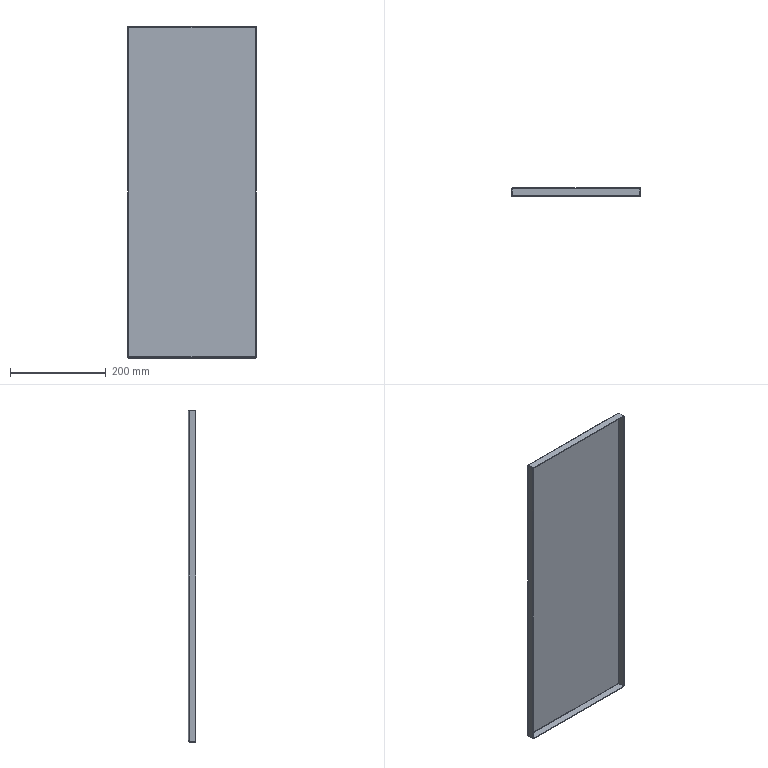Part | SolidWorks | features EdgeFlange 1, FlatPattern 1, SMBaseFlange 1, SheetMetal 1 | 1 solid | 38 faces | box 270 x 16.5 x 695 mm | volume 322735 mm3 | plane 22 | spline 8 | cylinder 8 | commonest cylinder face diameters 1.473 x4 4.473 x4
STEP:
#1=CARTESIAN_POINT('',(30.219,572.,-345.263));
#2=VERTEX_POINT('',#1);
#3=CARTESIAN_POINT('',(30.219,572.,345.263));
#4=VERTEX_POINT('',#3);
#5=CARTESIAN_POINT('',(30.219,572.,-345.788));
#6=DIRECTION('',(0.,0.,1.));
#7=VECTOR('',#6,1000.);
#8=LINE('',#5,#7);
#9=EDGE_CURVE('',#2,#4,#8,.T.);
#10=ORIENTED_EDGE('',*,*,#9,.F.);
#11=CARTESIAN_POINT('',(295.746,572.,-345.263));
#12=VERTEX_POINT('',#11);
#13=CARTESIAN_POINT('',(296.271,572.,-345.263));
#14=DIRECTION('',(-1.,0.,0.));
#15=VECTOR('',#14,1000.);
#16=LINE('',#13,#15);
#17=EDGE_CURVE('',#12,#2,#16,.T.);
#18=ORIENTED_EDGE('',*,*,#17,.F.);
#19=CARTESIAN_POINT('',(295.746,572.,345.263));
#20=VERTEX_POINT('',#19);
#21=CARTESIAN_POINT('',(295.746,572.,345.788));
#22=DIRECTION('',(0.,0.,-1.));
#23=VECTOR('',#22,1000.);
#24=LINE('',#21,#23);
#25=EDGE_CURVE('',#20,#12,#24,.T.);
#26=ORIENTED_EDGE('',*,*,#25,.F.);
#27=CARTESIAN_POINT('',(29.695,572.,345.263));
#28=DIRECTION('',(1.,0.,0.));
#29=VECTOR('',#28,1000.);
#30=LINE('',#27,#29);
#31=EDGE_CURVE('',#4,#20,#30,.T.);
#32=ORIENTED_EDGE('',*,*,#31,.F.);
#33=EDGE_LOOP('',(#10,#18,#26,#32));
#34=FACE_OUTER_BOUND('',#33,.T.);
#35=CARTESIAN_POINT('',(27.983,572.,347.5));
#36=DIRECTION('',(0.,1.,0.));
#37=DIRECTION('',(-1.,0.,0.));
#38=AXIS2_PLACEMENT_3D('',#35,#36,#37);
#39=PLANE('',#38);
#40=ADVANCED_FACE('',(#34),#39,.F.);
#41=CARTESIAN_POINT('',(295.746,573.5,-345.263));
#42=VERTEX_POINT('',#41);
#43=CARTESIAN_POINT('',(30.219,573.5,-345.263));
#44=VERTEX_POINT('',#43);
#45=CARTESIAN_POINT('',(296.271,573.5,-345.263));
#46=DIRECTION('',(-1.,0.,0.));
#47=VECTOR('',#46,1000.);
#48=LINE('',#45,#47);
#49=EDGE_CURVE('',#42,#44,#48,.T.);
#50=ORIENTED_EDGE('',*,*,#49,.T.);
#51=CARTESIAN_POINT('',(30.219,573.5,345.263));
#52=VERTEX_POINT('',#51);
#53=CARTESIAN_POINT('',(30.219,573.5,-345.788));
#54=DIRECTION('',(0.,0.,1.));
#55=VECTOR('',#54,1000.);
#56=LINE('',#53,#55);
#57=EDGE_CURVE('',#44,#52,#56,.T.);
#58=ORIENTED_EDGE('',*,*,#57,.T.);
#59=CARTESIAN_POINT('',(295.746,573.5,345.263));
#60=VERTEX_POINT('',#59);
#61=CARTESIAN_POINT('',(29.695,573.5,345.263));
#62=DIRECTION('',(1.,0.,0.));
#63=VECTOR('',#62,1000.);
#64=LINE('',#61,#63);
#65=EDGE_CURVE('',#52,#60,#64,.T.);
#66=ORIENTED_EDGE('',*,*,#65,.T.);
#67=CARTESIAN_POINT('',(295.746,573.5,345.788));
#68=DIRECTION('',(0.,0.,-1.));
#69=VECTOR('',#68,1000.);
#70=LINE('',#67,#69);
#71=EDGE_CURVE('',#60,#42,#70,.T.);
#72=ORIENTED_EDGE('',*,*,#71,.T.);
#73=EDGE_LOOP('',(#50,#58,#66,#72));
#74=FACE_OUTER_BOUND('',#73,.T.);
#75=CARTESIAN_POINT('',(27.983,573.5,347.5));
#76=DIRECTION('',(0.,1.,0.));
#77=DIRECTION('',(-1.,0.,0.));
#78=AXIS2_PLACEMENT_3D('',#75,#76,#77);
#79=PLANE('',#78);
#80=ADVANCED_FACE('',(#74),#79,.T.);
#81=CARTESIAN_POINT('',(296.271,571.263,347.5));
#82=VERTEX_POINT('',#81);
#83=CARTESIAN_POINT('',(296.271,571.263,346.));
#84=VERTEX_POINT('',#83);
#85=CARTESIAN_POINT('',(296.271,571.263,346.));
#86=DIRECTION('',(0.,0.,-1.));
#87=VECTOR('',#86,1000.);
#88=LINE('',#85,#87);
#89=EDGE_CURVE('',#82,#84,#88,.T.);
#90=ORIENTED_EDGE('',*,*,#89,.T.);
#91=CARTESIAN_POINT('',(295.746,572.,345.263));
#92=CARTESIAN_POINT('',(295.834,572.,345.456));
#93=CARTESIAN_POINT('',(295.921,571.921,345.648));
#94=CARTESIAN_POINT('',(296.096,571.648,345.921));
#95=CARTESIAN_POINT('',(296.183,571.456,346.));
#96=CARTESIAN_POINT('',(296.271,571.263,346.));
#97=B_SPLINE_CURVE_WITH_KNOTS('',3,(#91,#92,#93,#94,#95,#96),.UNSPECIFIED.,.F.,.F.,(4,2,4),(0.,0.5,1.),.UNSPECIFIED.);
#98=EDGE_CURVE('',#20,#84,#97,.T.);
#99=ORIENTED_EDGE('',*,*,#98,.F.);
#100=CARTESIAN_POINT('',(295.746,572.,345.263));
#101=DIRECTION('',(0.,1.,0.));
#102=VECTOR('',#101,1000.);
#103=LINE('',#100,#102);
#104=EDGE_CURVE('',#20,#60,#103,.T.);
#105=ORIENTED_EDGE('',*,*,#104,.T.);
#106=CARTESIAN_POINT('',(295.746,573.5,345.263));
#107=CARTESIAN_POINT('',(295.79,573.5,345.556));
#108=CARTESIAN_POINT('',(295.834,573.442,345.849));
#109=CARTESIAN_POINT('',(295.921,573.218,346.39));
#110=CARTESIAN_POINT('',(295.965,573.052,346.638));
#111=CARTESIAN_POINT('',(296.052,572.638,347.052));
#112=CARTESIAN_POINT('',(296.096,572.39,347.218));
#113=CARTESIAN_POINT('',(296.183,571.849,347.442));
#114=CARTESIAN_POINT('',(296.227,571.556,347.5));
#115=CARTESIAN_POINT('',(296.271,571.263,347.5));
#116=B_SPLINE_CURVE_WITH_KNOTS('',3,(#106,#107,#108,#109,#110,#111,#112,#113,#114,#115),.UNSPECIFIED.,.F.,.F.,(4,2,2,2,4),(0.,0.25,0.5,0.75,1.),.UNSPECIFIED.);
#117=EDGE_CURVE('',#60,#82,#116,.T.);
#118=ORIENTED_EDGE('',*,*,#117,.T.);
#119=EDGE_LOOP('',(#90,#99,#105,#118));
#120=FACE_OUTER_BOUND('',#119,.T.);
#121=CARTESIAN_POINT('',(295.746,573.515,345.263));
#122=CARTESIAN_POINT('',(295.79,573.515,345.558));
#123=CARTESIAN_POINT('',(295.834,573.456,345.853));
#124=CARTESIAN_POINT('',(295.921,573.231,346.397));
#125=CARTESIAN_POINT('',(295.965,573.064,346.647));
#126=CARTESIAN_POINT('',(296.052,572.647,347.064));
#127=CARTESIAN_POINT('',(296.096,572.397,347.231));
#128=CARTESIAN_POINT('',(296.183,571.853,347.456));
#129=CARTESIAN_POINT('',(296.227,571.558,347.515));
#130=CARTESIAN_POINT('',(296.271,571.263,347.515));
#131=CARTESIAN_POINT('',(295.746,573.5,345.263));
#132=CARTESIAN_POINT('',(295.79,573.5,345.556));
#133=CARTESIAN_POINT('',(295.834,573.442,345.849));
#134=CARTESIAN_POINT('',(295.921,573.218,346.39));
#135=CARTESIAN_POINT('',(295.965,573.052,346.638));
#136=CARTESIAN_POINT('',(296.052,572.638,347.052));
#137=CARTESIAN_POINT('',(296.096,572.39,347.218));
#138=CARTESIAN_POINT('',(296.183,571.849,347.442));
#139=CARTESIAN_POINT('',(296.227,571.556,347.5));
#140=CARTESIAN_POINT('',(296.271,571.263,347.5));
#141=CARTESIAN_POINT('',(295.746,572.,345.263));
#142=CARTESIAN_POINT('',(295.79,572.,345.36));
#143=CARTESIAN_POINT('',(295.834,571.981,345.456));
#144=CARTESIAN_POINT('',(295.921,571.907,345.634));
#145=CARTESIAN_POINT('',(295.965,571.852,345.716));
#146=CARTESIAN_POINT('',(296.052,571.716,345.852));
#147=CARTESIAN_POINT('',(296.096,571.634,345.907));
#148=CARTESIAN_POINT('',(296.183,571.456,345.981));
#149=CARTESIAN_POINT('',(296.227,571.36,346.));
#150=CARTESIAN_POINT('',(296.271,571.263,346.));
#151=CARTESIAN_POINT('',(295.746,571.985,345.263));
#152=CARTESIAN_POINT('',(295.79,571.985,345.358));
#153=CARTESIAN_POINT('',(295.834,571.966,345.452));
#154=CARTESIAN_POINT('',(295.921,571.894,345.627));
#155=CARTESIAN_POINT('',(295.965,571.84,345.707));
#156=CARTESIAN_POINT('',(296.052,571.707,345.84));
#157=CARTESIAN_POINT('',(296.096,571.627,345.894));
#158=CARTESIAN_POINT('',(296.183,571.452,345.966));
#159=CARTESIAN_POINT('',(296.227,571.358,345.985));
#160=CARTESIAN_POINT('',(296.271,571.263,345.985));
#161=B_SPLINE_SURFACE_WITH_KNOTS('',1,3,((#121,#122,#123,#124,#125,#126,#127,#128,#129,#130),(#131,#132,#133,#134,#135,#136,#137,#138,#139,#140),(#141,#142,#143,#144,#145,#146,#147,#148,#149,#150),(#151,#152,#153,#154,#155,#156,#157,#158,#159,#160)),.UNSPECIFIED.,.F.,.F.,.F.,(2,1,1,2),(4,2,2,2,4),(-0.01,0.,1.,1.01),(0.,0.25,0.5,0.75,1.),.UNSPECIFIED.);
#162=ADVANCED_FACE('',(#120),#161,.F.);
#163=CARTESIAN_POINT('',(29.695,571.263,346.));
#164=VERTEX_POINT('',#163);
#165=CARTESIAN_POINT('',(29.695,571.263,346.));
#166=CARTESIAN_POINT('',(29.782,571.456,346.));
#167=CARTESIAN_POINT('',(29.87,571.648,345.921));
#168=CARTESIAN_POINT('',(30.045,571.921,345.648));
#169=CARTESIAN_POINT('',(30.132,572.,345.456));
#170=CARTESIAN_POINT('',(30.219,572.,345.263));
#171=B_SPLINE_CURVE_WITH_KNOTS('',3,(#165,#166,#167,#168,#169,#170),.UNSPECIFIED.,.F.,.F.,(4,2,4),(0.,0.5,1.),.UNSPECIFIED.);
#172=EDGE_CURVE('',#164,#4,#171,.T.);
#173=ORIENTED_EDGE('',*,*,#172,.F.);
#174=CARTESIAN_POINT('',(29.695,571.263,347.5));
#175=VERTEX_POINT('',#174);
#176=CARTESIAN_POINT('',(29.695,571.263,346.));
#177=DIRECTION('',(0.,0.,-1.));
#178=VECTOR('',#177,1000.);
#179=LINE('',#176,#178);
#180=EDGE_CURVE('',#175,#164,#179,.T.);
#181=ORIENTED_EDGE('',*,*,#180,.F.);
#182=CARTESIAN_POINT('',(29.695,571.263,347.5));
#183=CARTESIAN_POINT('',(29.739,571.556,347.5));
#184=CARTESIAN_POINT('',(29.782,571.849,347.442));
#185=CARTESIAN_POINT('',(29.87,572.39,347.218));
#186=CARTESIAN_POINT('',(29.913,572.638,347.052));
#187=CARTESIAN_POINT('',(30.001,573.052,346.638));
#188=CARTESIAN_POINT('',(30.045,573.218,346.39));
#189=CARTESIAN_POINT('',(30.132,573.442,345.849));
#190=CARTESIAN_POINT('',(30.176,573.5,345.556));
#191=CARTESIAN_POINT('',(30.219,573.5,345.263));
#192=B_SPLINE_CURVE_WITH_KNOTS('',3,(#182,#183,#184,#185,#186,#187,#188,#189,#190,#191),.UNSPECIFIED.,.F.,.F.,(4,2,2,2,4),(0.,0.25,0.5,0.75,1.),.UNSPECIFIED.);
#193=EDGE_CURVE('',#175,#52,#192,.T.);
#194=ORIENTED_EDGE('',*,*,#193,.T.);
#195=CARTESIAN_POINT('',(30.219,572.,345.263));
#196=DIRECTION('',(0.,1.,0.));
#197=VECTOR('',#196,1000.);
#198=LINE('',#195,#197);
#199=EDGE_CURVE('',#4,#52,#198,.T.);
#200=ORIENTED_EDGE('',*,*,#199,.F.);
#201=EDGE_LOOP('',(#173,#181,#194,#200));
#202=FACE_OUTER_BOUND('',#201,.T.);
#203=CARTESIAN_POINT('',(29.695,571.263,347.515));
#204=CARTESIAN_POINT('',(29.739,571.558,347.515));
#205=CARTESIAN_POINT('',(29.782,571.853,347.456));
#206=CARTESIAN_POINT('',(29.87,572.397,347.231));
#207=CARTESIAN_POINT('',(29.913,572.647,347.064));
#208=CARTESIAN_POINT('',(30.001,573.064,346.647));
#209=CARTESIAN_POINT('',(30.045,573.231,346.397));
#210=CARTESIAN_POINT('',(30.132,573.456,345.853));
#211=CARTESIAN_POINT('',(30.176,573.515,345.558));
#212=CARTESIAN_POINT('',(30.219,573.515,345.263));
#213=CARTESIAN_POINT('',(29.695,571.263,347.5));
#214=CARTESIAN_POINT('',(29.739,571.556,347.5));
#215=CARTESIAN_POINT('',(29.782,571.849,347.442));
#216=CARTESIAN_POINT('',(29.87,572.39,347.218));
#217=CARTESIAN_POINT('',(29.913,572.638,347.052));
#218=CARTESIAN_POINT('',(30.001,573.052,346.638));
#219=CARTESIAN_POINT('',(30.045,573.218,346.39));
#220=CARTESIAN_POINT('',(30.132,573.442,345.849));
#221=CARTESIAN_POINT('',(30.176,573.5,345.556));
#222=CARTESIAN_POINT('',(30.219,573.5,345.263));
#223=CARTESIAN_POINT('',(29.695,571.263,346.));
#224=CARTESIAN_POINT('',(29.739,571.36,346.));
#225=CARTESIAN_POINT('',(29.782,571.456,345.981));
#226=CARTESIAN_POINT('',(29.87,571.634,345.907));
#227=CARTESIAN_POINT('',(29.913,571.716,345.852));
#228=CARTESIAN_POINT('',(30.001,571.852,345.716));
#229=CARTESIAN_POINT('',(30.045,571.907,345.634));
#230=CARTESIAN_POINT('',(30.132,571.981,345.456));
#231=CARTESIAN_POINT('',(30.176,572.,345.36));
#232=CARTESIAN_POINT('',(30.219,572.,345.263));
#233=CARTESIAN_POINT('',(29.695,571.263,345.985));
#234=CARTESIAN_POINT('',(29.739,571.358,345.985));
#235=CARTESIAN_POINT('',(29.782,571.452,345.966));
#236=CARTESIAN_POINT('',(29.87,571.627,345.894));
#237=CARTESIAN_POINT('',(29.913,571.707,345.84));
#238=CARTESIAN_POINT('',(30.001,571.84,345.707));
#239=CARTESIAN_POINT('',(30.045,571.894,345.627));
#240=CARTESIAN_POINT('',(30.132,571.966,345.452));
#241=CARTESIAN_POINT('',(30.176,571.985,345.358));
#242=CARTESIAN_POINT('',(30.219,571.985,345.263));
#243=B_SPLINE_SURFACE_WITH_KNOTS('',1,3,((#203,#204,#205,#206,#207,#208,#209,#210,#211,#212),(#213,#214,#215,#216,#217,#218,#219,#220,#221,#222),(#223,#224,#225,#226,#227,#228,#229,#230,#231,#232),(#233,#234,#235,#236,#237,#238,#239,#240,#241,#242)),.UNSPECIFIED.,.F.,.F.,.F.,(2,1,1,2),(4,2,2,2,4),(-0.01,0.,1.,1.01),(0.,0.25,0.5,0.75,1.),.UNSPECIFIED.);
#244=ADVANCED_FACE('',(#202),#243,.F.);
#245=ORIENTED_EDGE('',*,*,#65,.F.);
#246=ORIENTED_EDGE('',*,*,#193,.F.);
#247=CARTESIAN_POINT('',(0.,571.263,347.5));
#248=DIRECTION('',(-1.,0.,0.));
#249=VECTOR('',#248,1000.);
#250=LINE('',#247,#249);
#251=EDGE_CURVE('',#82,#175,#250,.T.);
#252=ORIENTED_EDGE('',*,*,#251,.F.);
#253=ORIENTED_EDGE('',*,*,#117,.F.);
#254=EDGE_LOOP('',(#245,#246,#252,#253));
#255=FACE_OUTER_BOUND('',#254,.T.);
#256=CARTESIAN_POINT('',(29.695,571.263,345.263));
#257=DIRECTION('',(-1.,0.,0.));
#258=DIRECTION('',(0.,0.,1.));
#259=AXIS2_PLACEMENT_3D('',#256,#257,#258);
#260=CYLINDRICAL_SURFACE('',#259,2.237);
#261=ADVANCED_FACE('',(#255),#260,.T.);
#262=ORIENTED_EDGE('',*,*,#31,.T.);
#263=ORIENTED_EDGE('',*,*,#98,.T.);
#264=CARTESIAN_POINT('',(297.983,571.263,346.));
#265=DIRECTION('',(-1.,0.,0.));
#266=VECTOR('',#265,1000.);
#267=LINE('',#264,#266);
#268=EDGE_CURVE('',#84,#164,#267,.T.);
#269=ORIENTED_EDGE('',*,*,#268,.T.);
#270=ORIENTED_EDGE('',*,*,#172,.T.);
#271=EDGE_LOOP('',(#262,#263,#269,#270));
#272=FACE_OUTER_BOUND('',#271,.T.);
#273=CARTESIAN_POINT('',(29.695,571.263,345.263));
#274=DIRECTION('',(-1.,0.,0.));
#275=DIRECTION('',(0.,0.,1.));
#276=AXIS2_PLACEMENT_3D('',#273,#274,#275);
#277=CYLINDRICAL_SURFACE('',#276,0.7366);
#278=ADVANCED_FACE('',(#272),#277,.F.);
#279=CARTESIAN_POINT('',(296.271,557.,346.));
#280=VERTEX_POINT('',#279);
#281=CARTESIAN_POINT('',(296.271,557.,347.5));
#282=VERTEX_POINT('',#281);
#283=CARTESIAN_POINT('',(296.271,557.,347.5));
#284=DIRECTION('',(0.,0.,1.));
#285=VECTOR('',#284,1000.);
#286=LINE('',#283,#285);
#287=EDGE_CURVE('',#280,#282,#286,.T.);
#288=ORIENTED_EDGE('',*,*,#287,.F.);
#289=CARTESIAN_POINT('',(296.271,0.,346.));
#290=DIRECTION('',(0.,-1.,0.));
#291=VECTOR('',#290,1000.);
#292=LINE('',#289,#291);
#293=EDGE_CURVE('',#84,#280,#292,.T.);
#294=ORIENTED_EDGE('',*,*,#293,.F.);
#295=ORIENTED_EDGE('',*,*,#89,.F.);
#296=CARTESIAN_POINT('',(296.271,0.,347.5));
#297=DIRECTION('',(0.,1.,0.));
#298=VECTOR('',#297,1000.);
#299=LINE('',#296,#298);
#300=EDGE_CURVE('',#282,#82,#299,.T.);
#301=ORIENTED_EDGE('',*,*,#300,.F.);
#302=EDGE_LOOP('',(#288,#294,#295,#301));
#303=FACE_OUTER_BOUND('',#302,.T.);
#304=CARTESIAN_POINT('',(296.271,572.,346.));
#305=DIRECTION('',(1.,0.,0.));
#306=DIRECTION('',(0.,1.,0.));
#307=AXIS2_PLACEMENT_3D('',#304,#305,#306);
#308=PLANE('',#307);
#309=ADVANCED_FACE('',(#303),#308,.T.);
#310=CARTESIAN_POINT('',(29.695,557.,347.5));
#311=VERTEX_POINT('',#310);
#312=CARTESIAN_POINT('',(29.695,572.,347.5));
#313=DIRECTION('',(0.,1.,0.));
#314=VECTOR('',#313,1000.);
#315=LINE('',#312,#314);
#316=EDGE_CURVE('',#311,#175,#315,.T.);
#317=ORIENTED_EDGE('',*,*,#316,.F.);
#318=CARTESIAN_POINT('',(27.983,557.,347.5));
#319=DIRECTION('',(-1.,0.,0.));
#320=VECTOR('',#319,1000.);
#321=LINE('',#318,#320);
#322=EDGE_CURVE('',#282,#311,#321,.T.);
#323=ORIENTED_EDGE('',*,*,#322,.F.);
#324=ORIENTED_EDGE('',*,*,#300,.T.);
#325=ORIENTED_EDGE('',*,*,#251,.T.);
#326=EDGE_LOOP('',(#317,#323,#324,#325));
#327=FACE_OUTER_BOUND('',#326,.T.);
#328=CARTESIAN_POINT('',(0.,0.,347.5));
#329=DIRECTION('',(0.,0.,1.));
#330=DIRECTION('',(0.,-1.,0.));
#331=AXIS2_PLACEMENT_3D('',#328,#329,#330);
#332=PLANE('',#331);
#333=ADVANCED_FACE('',(#327),#332,.T.);
#334=CARTESIAN_POINT('',(29.695,557.,346.));
#335=VERTEX_POINT('',#334);
#336=CARTESIAN_POINT('',(0.,557.,346.));
#337=DIRECTION('',(-1.,0.,0.));
#338=VECTOR('',#337,1000.);
#339=LINE('',#336,#338);
#340=EDGE_CURVE('',#280,#335,#339,.T.);
#341=ORIENTED_EDGE('',*,*,#340,.T.);
#342=CARTESIAN_POINT('',(29.695,572.,346.));
#343=DIRECTION('',(0.,-1.,0.));
#344=VECTOR('',#343,1000.);
#345=LINE('',#342,#344);
#346=EDGE_CURVE('',#164,#335,#345,.T.);
#347=ORIENTED_EDGE('',*,*,#346,.F.);
#348=ORIENTED_EDGE('',*,*,#268,.F.);
#349=ORIENTED_EDGE('',*,*,#293,.T.);
#350=EDGE_LOOP('',(#341,#347,#348,#349));
#351=FACE_OUTER_BOUND('',#350,.T.);
#352=CARTESIAN_POINT('',(0.,0.,346.));
#353=DIRECTION('',(0.,0.,1.));
#354=DIRECTION('',(0.,-1.,0.));
#355=AXIS2_PLACEMENT_3D('',#352,#353,#354);
#356=PLANE('',#355);
#357=ADVANCED_FACE('',(#351),#356,.F.);
#358=CARTESIAN_POINT('',(29.695,557.,346.));
#359=DIRECTION('',(0.,0.,1.));
#360=VECTOR('',#359,1000.);
#361=LINE('',#358,#360);
#362=EDGE_CURVE('',#335,#311,#361,.T.);
#363=ORIENTED_EDGE('',*,*,#362,.F.);
#364=ORIENTED_EDGE('',*,*,#340,.F.);
#365=ORIENTED_EDGE('',*,*,#287,.T.);
#366=ORIENTED_EDGE('',*,*,#322,.T.);
#367=EDGE_LOOP('',(#363,#364,#365,#366));
#368=FACE_OUTER_BOUND('',#367,.T.);
#369=CARTESIAN_POINT('',(27.983,557.,347.5));
#370=DIRECTION('',(0.,-1.,0.));
#371=DIRECTION('',(0.,0.,-1.));
#372=AXIS2_PLACEMENT_3D('',#369,#370,#371);
#373=PLANE('',#372);
#374=ADVANCED_FACE('',(#368),#373,.T.);
#375=ORIENTED_EDGE('',*,*,#346,.T.);
#376=ORIENTED_EDGE('',*,*,#362,.T.);
#377=ORIENTED_EDGE('',*,*,#316,.T.);
#378=ORIENTED_EDGE('',*,*,#180,.T.);
#379=EDGE_LOOP('',(#375,#376,#377,#378));
#380=FACE_OUTER_BOUND('',#379,.T.);
#381=CARTESIAN_POINT('',(29.695,572.,346.));
#382=DIRECTION('',(1.,0.,0.));
#383=DIRECTION('',(0.,1.,0.));
#384=AXIS2_PLACEMENT_3D('',#381,#382,#383);
#385=PLANE('',#384);
#386=ADVANCED_FACE('',(#380),#385,.F.);
#387=CARTESIAN_POINT('',(297.983,571.263,-345.788));
#388=VERTEX_POINT('',#387);
#389=CARTESIAN_POINT('',(296.483,571.263,-345.788));
#390=VERTEX_POINT('',#389);
#391=CARTESIAN_POINT('',(296.483,571.263,-345.788));
#392=DIRECTION('',(-1.,0.,0.));
#393=VECTOR('',#392,1000.);
#394=LINE('',#391,#393);
#395=EDGE_CURVE('',#388,#390,#394,.T.);
#396=ORIENTED_EDGE('',*,*,#395,.T.);
#397=CARTESIAN_POINT('',(295.746,572.,-345.263));
#398=CARTESIAN_POINT('',(295.939,572.,-345.351));
#399=CARTESIAN_POINT('',(296.131,571.921,-345.438));
#400=CARTESIAN_POINT('',(296.403,571.648,-345.613));
#401=CARTESIAN_POINT('',(296.483,571.456,-345.7));
#402=CARTESIAN_POINT('',(296.483,571.263,-345.788));
#403=B_SPLINE_CURVE_WITH_KNOTS('',3,(#397,#398,#399,#400,#401,#402),.UNSPECIFIED.,.F.,.F.,(4,2,4),(0.,0.5,1.),.UNSPECIFIED.);
#404=EDGE_CURVE('',#12,#390,#403,.T.);
#405=ORIENTED_EDGE('',*,*,#404,.F.);
#406=CARTESIAN_POINT('',(295.746,572.,-345.263));
#407=DIRECTION('',(0.,1.,0.));
#408=VECTOR('',#407,1000.);
#409=LINE('',#406,#408);
#410=EDGE_CURVE('',#12,#42,#409,.T.);
#411=ORIENTED_EDGE('',*,*,#410,.T.);
#412=CARTESIAN_POINT('',(295.746,573.5,-345.263));
#413=CARTESIAN_POINT('',(296.039,573.5,-345.307));
#414=CARTESIAN_POINT('',(296.332,573.442,-345.351));
#415=CARTESIAN_POINT('',(296.873,573.218,-345.438));
#416=CARTESIAN_POINT('',(297.121,573.052,-345.482));
#417=CARTESIAN_POINT('',(297.535,572.638,-345.569));
#418=CARTESIAN_POINT('',(297.701,572.39,-345.613));
#419=CARTESIAN_POINT('',(297.925,571.849,-345.7));
#420=CARTESIAN_POINT('',(297.983,571.556,-345.744));
#421=CARTESIAN_POINT('',(297.983,571.263,-345.788));
#422=B_SPLINE_CURVE_WITH_KNOTS('',3,(#412,#413,#414,#415,#416,#417,#418,#419,#420,#421),.UNSPECIFIED.,.F.,.F.,(4,2,2,2,4),(0.,0.25,0.5,0.75,1.),.UNSPECIFIED.);
#423=EDGE_CURVE('',#42,#388,#422,.T.);
#424=ORIENTED_EDGE('',*,*,#423,.T.);
#425=EDGE_LOOP('',(#396,#405,#411,#424));
#426=FACE_OUTER_BOUND('',#425,.T.);
#427=CARTESIAN_POINT('',(295.746,573.515,-345.263));
#428=CARTESIAN_POINT('',(296.041,573.515,-345.307));
#429=CARTESIAN_POINT('',(296.336,573.456,-345.351));
#430=CARTESIAN_POINT('',(296.88,573.231,-345.438));
#431=CARTESIAN_POINT('',(297.13,573.064,-345.482));
#432=CARTESIAN_POINT('',(297.547,572.647,-345.569));
#433=CARTESIAN_POINT('',(297.714,572.397,-345.613));
#434=CARTESIAN_POINT('',(297.939,571.853,-345.7));
#435=CARTESIAN_POINT('',(297.998,571.558,-345.744));
#436=CARTESIAN_POINT('',(297.998,571.263,-345.788));
#437=CARTESIAN_POINT('',(295.746,573.5,-345.263));
#438=CARTESIAN_POINT('',(296.039,573.5,-345.307));
#439=CARTESIAN_POINT('',(296.332,573.442,-345.351));
#440=CARTESIAN_POINT('',(296.873,573.218,-345.438));
#441=CARTESIAN_POINT('',(297.121,573.052,-345.482));
#442=CARTESIAN_POINT('',(297.535,572.638,-345.569));
#443=CARTESIAN_POINT('',(297.701,572.39,-345.613));
#444=CARTESIAN_POINT('',(297.925,571.849,-345.7));
#445=CARTESIAN_POINT('',(297.983,571.556,-345.744));
#446=CARTESIAN_POINT('',(297.983,571.263,-345.788));
#447=CARTESIAN_POINT('',(295.746,572.,-345.263));
#448=CARTESIAN_POINT('',(295.843,572.,-345.307));
#449=CARTESIAN_POINT('',(295.939,571.981,-345.351));
#450=CARTESIAN_POINT('',(296.117,571.907,-345.438));
#451=CARTESIAN_POINT('',(296.199,571.852,-345.482));
#452=CARTESIAN_POINT('',(296.335,571.716,-345.569));
#453=CARTESIAN_POINT('',(296.39,571.634,-345.613));
#454=CARTESIAN_POINT('',(296.464,571.456,-345.7));
#455=CARTESIAN_POINT('',(296.483,571.36,-345.744));
#456=CARTESIAN_POINT('',(296.483,571.263,-345.788));
#457=CARTESIAN_POINT('',(295.746,571.985,-345.263));
#458=CARTESIAN_POINT('',(295.841,571.985,-345.307));
#459=CARTESIAN_POINT('',(295.935,571.966,-345.351));
#460=CARTESIAN_POINT('',(296.11,571.894,-345.438));
#461=CARTESIAN_POINT('',(296.19,571.84,-345.482));
#462=CARTESIAN_POINT('',(296.323,571.707,-345.569));
#463=CARTESIAN_POINT('',(296.377,571.627,-345.613));
#464=CARTESIAN_POINT('',(296.449,571.452,-345.7));
#465=CARTESIAN_POINT('',(296.468,571.358,-345.744));
#466=CARTESIAN_POINT('',(296.468,571.263,-345.788));
#467=B_SPLINE_SURFACE_WITH_KNOTS('',1,3,((#427,#428,#429,#430,#431,#432,#433,#434,#435,#436),(#437,#438,#439,#440,#441,#442,#443,#444,#445,#446),(#447,#448,#449,#450,#451,#452,#453,#454,#455,#456),(#457,#458,#459,#460,#461,#462,#463,#464,#465,#466)),.UNSPECIFIED.,.F.,.F.,.F.,(2,1,1,2),(4,2,2,2,4),(-0.01,0.,1.,1.01),(0.,0.25,0.5,0.75,1.),.UNSPECIFIED.);
#468=ADVANCED_FACE('',(#426),#467,.F.);
#469=CARTESIAN_POINT('',(296.483,571.263,345.788));
#470=VERTEX_POINT('',#469);
#471=CARTESIAN_POINT('',(296.483,571.263,345.788));
#472=CARTESIAN_POINT('',(296.483,571.456,345.7));
#473=CARTESIAN_POINT('',(296.403,571.648,345.613));
#474=CARTESIAN_POINT('',(296.131,571.921,345.438));
#475=CARTESIAN_POINT('',(295.939,572.,345.351));
#476=CARTESIAN_POINT('',(295.746,572.,345.263));
#477=B_SPLINE_CURVE_WITH_KNOTS('',3,(#471,#472,#473,#474,#475,#476),.UNSPECIFIED.,.F.,.F.,(4,2,4),(0.,0.5,1.),.UNSPECIFIED.);
#478=EDGE_CURVE('',#470,#20,#477,.T.);
#479=ORIENTED_EDGE('',*,*,#478,.F.);
#480=CARTESIAN_POINT('',(297.983,571.263,345.788));
#481=VERTEX_POINT('',#480);
#482=CARTESIAN_POINT('',(296.483,571.263,345.788));
#483=DIRECTION('',(-1.,0.,0.));
#484=VECTOR('',#483,1000.);
#485=LINE('',#482,#484);
#486=EDGE_CURVE('',#481,#470,#485,.T.);
#487=ORIENTED_EDGE('',*,*,#486,.F.);
#488=CARTESIAN_POINT('',(297.983,571.263,345.788));
#489=CARTESIAN_POINT('',(297.983,571.556,345.744));
#490=CARTESIAN_POINT('',(297.925,571.849,345.7));
#491=CARTESIAN_POINT('',(297.701,572.39,345.613));
#492=CARTESIAN_POINT('',(297.535,572.638,345.569));
#493=CARTESIAN_POINT('',(297.121,573.052,345.482));
#494=CARTESIAN_POINT('',(296.873,573.218,345.438));
#495=CARTESIAN_POINT('',(296.332,573.442,345.351));
#496=CARTESIAN_POINT('',(296.039,573.5,345.307));
#497=CARTESIAN_POINT('',(295.746,573.5,345.263));
#498=B_SPLINE_CURVE_WITH_KNOTS('',3,(#488,#489,#490,#491,#492,#493,#494,#495,#496,#497),.UNSPECIFIED.,.F.,.F.,(4,2,2,2,4),(0.,0.25,0.5,0.75,1.),.UNSPECIFIED.);
#499=EDGE_CURVE('',#481,#60,#498,.T.);
#500=ORIENTED_EDGE('',*,*,#499,.T.);
#501=ORIENTED_EDGE('',*,*,#104,.F.);
#502=EDGE_LOOP('',(#479,#487,#500,#501));
#503=FACE_OUTER_BOUND('',#502,.T.);
#504=CARTESIAN_POINT('',(297.998,571.263,345.788));
#505=CARTESIAN_POINT('',(297.998,571.558,345.744));
#506=CARTESIAN_POINT('',(297.939,571.853,345.7));
#507=CARTESIAN_POINT('',(297.714,572.397,345.613));
#508=CARTESIAN_POINT('',(297.547,572.647,345.569));
#509=CARTESIAN_POINT('',(297.13,573.064,345.482));
#510=CARTESIAN_POINT('',(296.88,573.231,345.438));
#511=CARTESIAN_POINT('',(296.336,573.456,345.351));
#512=CARTESIAN_POINT('',(296.041,573.515,345.307));
#513=CARTESIAN_POINT('',(295.746,573.515,345.263));
#514=CARTESIAN_POINT('',(297.983,571.263,345.788));
#515=CARTESIAN_POINT('',(297.983,571.556,345.744));
#516=CARTESIAN_POINT('',(297.925,571.849,345.7));
#517=CARTESIAN_POINT('',(297.701,572.39,345.613));
#518=CARTESIAN_POINT('',(297.535,572.638,345.569));
#519=CARTESIAN_POINT('',(297.121,573.052,345.482));
#520=CARTESIAN_POINT('',(296.873,573.218,345.438));
#521=CARTESIAN_POINT('',(296.332,573.442,345.351));
#522=CARTESIAN_POINT('',(296.039,573.5,345.307));
#523=CARTESIAN_POINT('',(295.746,573.5,345.263));
#524=CARTESIAN_POINT('',(296.483,571.263,345.788));
#525=CARTESIAN_POINT('',(296.483,571.36,345.744));
#526=CARTESIAN_POINT('',(296.464,571.456,345.7));
#527=CARTESIAN_POINT('',(296.39,571.634,345.613));
#528=CARTESIAN_POINT('',(296.335,571.716,345.569));
#529=CARTESIAN_POINT('',(296.199,571.852,345.482));
#530=CARTESIAN_POINT('',(296.117,571.907,345.438));
#531=CARTESIAN_POINT('',(295.939,571.981,345.351));
#532=CARTESIAN_POINT('',(295.843,572.,345.307));
#533=CARTESIAN_POINT('',(295.746,572.,345.263));
#534=CARTESIAN_POINT('',(296.468,571.263,345.788));
#535=CARTESIAN_POINT('',(296.468,571.358,345.744));
#536=CARTESIAN_POINT('',(296.449,571.452,345.7));
#537=CARTESIAN_POINT('',(296.377,571.627,345.613));
#538=CARTESIAN_POINT('',(296.323,571.707,345.569));
#539=CARTESIAN_POINT('',(296.19,571.84,345.482));
#540=CARTESIAN_POINT('',(296.11,571.894,345.438));
#541=CARTESIAN_POINT('',(295.935,571.966,345.351));
#542=CARTESIAN_POINT('',(295.841,571.985,345.307));
#543=CARTESIAN_POINT('',(295.746,571.985,345.263));
#544=B_SPLINE_SURFACE_WITH_KNOTS('',1,3,((#504,#505,#506,#507,#508,#509,#510,#511,#512,#513),(#514,#515,#516,#517,#518,#519,#520,#521,#522,#523),(#524,#525,#526,#527,#528,#529,#530,#531,#532,#533),(#534,#535,#536,#537,#538,#539,#540,#541,#542,#543)),.UNSPECIFIED.,.F.,.F.,.F.,(2,1,1,2),(4,2,2,2,4),(-0.01,0.,1.,1.01),(0.,0.25,0.5,0.75,1.),.UNSPECIFIED.);
#545=ADVANCED_FACE('',(#503),#544,.F.);
#546=ORIENTED_EDGE('',*,*,#71,.F.);
#547=ORIENTED_EDGE('',*,*,#499,.F.);
#548=CARTESIAN_POINT('',(297.983,571.263,-347.5));
#549=DIRECTION('',(0.,0.,-1.));
#550=VECTOR('',#549,1000.);
#551=LINE('',#548,#550);
#552=EDGE_CURVE('',#481,#388,#551,.T.);
#553=ORIENTED_EDGE('',*,*,#552,.T.);
#554=ORIENTED_EDGE('',*,*,#423,.F.);
#555=EDGE_LOOP('',(#546,#547,#553,#554));
#556=FACE_OUTER_BOUND('',#555,.T.);
#557=CARTESIAN_POINT('',(295.746,571.263,345.788));
#558=DIRECTION('',(0.,0.,1.));
#559=DIRECTION('',(1.,0.,0.));
#560=AXIS2_PLACEMENT_3D('',#557,#558,#559);
#561=CYLINDRICAL_SURFACE('',#560,2.237);
#562=ADVANCED_FACE('',(#556),#561,.T.);
#563=ORIENTED_EDGE('',*,*,#25,.T.);
#564=ORIENTED_EDGE('',*,*,#404,.T.);
#565=CARTESIAN_POINT('',(296.483,571.263,-347.5));
#566=DIRECTION('',(0.,0.,1.));
#567=VECTOR('',#566,1000.);
#568=LINE('',#565,#567);
#569=EDGE_CURVE('',#390,#470,#568,.T.);
#570=ORIENTED_EDGE('',*,*,#569,.T.);
#571=ORIENTED_EDGE('',*,*,#478,.T.);
#572=EDGE_LOOP('',(#563,#564,#570,#571));
#573=FACE_OUTER_BOUND('',#572,.T.);
#574=CARTESIAN_POINT('',(295.746,571.263,345.788));
#575=DIRECTION('',(0.,0.,1.));
#576=DIRECTION('',(1.,0.,0.));
#577=AXIS2_PLACEMENT_3D('',#574,#575,#576);
#578=CYLINDRICAL_SURFACE('',#577,0.7366);
#579=ADVANCED_FACE('',(#573),#578,.F.);
#580=CARTESIAN_POINT('',(296.483,557.,-345.788));
#581=VERTEX_POINT('',#580);
#582=CARTESIAN_POINT('',(297.983,557.,-345.788));
#583=VERTEX_POINT('',#582);
#584=CARTESIAN_POINT('',(297.983,557.,-345.788));
#585=DIRECTION('',(1.,0.,0.));
#586=VECTOR('',#585,1000.);
#587=LINE('',#584,#586);
#588=EDGE_CURVE('',#581,#583,#587,.T.);
#589=ORIENTED_EDGE('',*,*,#588,.F.);
#590=CARTESIAN_POINT('',(296.483,0.,-345.788));
#591=DIRECTION('',(0.,-1.,0.));
#592=VECTOR('',#591,1000.);
#593=LINE('',#590,#592);
#594=EDGE_CURVE('',#390,#581,#593,.T.);
#595=ORIENTED_EDGE('',*,*,#594,.F.);
#596=ORIENTED_EDGE('',*,*,#395,.F.);
#597=CARTESIAN_POINT('',(297.983,572.,-345.788));
#598=DIRECTION('',(0.,-1.,0.));
#599=VECTOR('',#598,1000.);
#600=LINE('',#597,#599);
#601=EDGE_CURVE('',#388,#583,#600,.T.);
#602=ORIENTED_EDGE('',*,*,#601,.T.);
#603=EDGE_LOOP('',(#589,#595,#596,#602));
#604=FACE_OUTER_BOUND('',#603,.T.);
#605=CARTESIAN_POINT('',(296.483,572.,-345.788));
#606=DIRECTION('',(0.,0.,-1.));
#607=DIRECTION('',(0.,1.,0.));
#608=AXIS2_PLACEMENT_3D('',#605,#606,#607);
#609=PLANE('',#608);
#610=ADVANCED_FACE('',(#604),#609,.T.);
#611=ORIENTED_EDGE('',*,*,#552,.F.);
#612=CARTESIAN_POINT('',(297.983,557.,345.788));
#613=VERTEX_POINT('',#612);
#614=CARTESIAN_POINT('',(297.983,0.,345.788));
#615=DIRECTION('',(0.,-1.,0.));
#616=VECTOR('',#615,1000.);
#617=LINE('',#614,#616);
#618=EDGE_CURVE('',#481,#613,#617,.T.);
#619=ORIENTED_EDGE('',*,*,#618,.T.);
#620=CARTESIAN_POINT('',(297.983,557.,-347.5));
#621=DIRECTION('',(0.,0.,1.));
#622=VECTOR('',#621,1000.);
#623=LINE('',#620,#622);
#624=EDGE_CURVE('',#583,#613,#623,.T.);
#625=ORIENTED_EDGE('',*,*,#624,.F.);
#626=ORIENTED_EDGE('',*,*,#601,.F.);
#627=EDGE_LOOP('',(#611,#619,#625,#626));
#628=FACE_OUTER_BOUND('',#627,.T.);
#629=CARTESIAN_POINT('',(297.983,0.,0.));
#630=DIRECTION('',(-1.,0.,0.));
#631=DIRECTION('',(0.,-1.,0.));
#632=AXIS2_PLACEMENT_3D('',#629,#630,#631);
#633=PLANE('',#632);
#634=ADVANCED_FACE('',(#628),#633,.F.);
#635=CARTESIAN_POINT('',(296.483,557.,345.788));
#636=VERTEX_POINT('',#635);
#637=CARTESIAN_POINT('',(296.483,572.,345.788));
#638=DIRECTION('',(0.,-1.,0.));
#639=VECTOR('',#638,1000.);
#640=LINE('',#637,#639);
#641=EDGE_CURVE('',#470,#636,#640,.T.);
#642=ORIENTED_EDGE('',*,*,#641,.F.);
#643=ORIENTED_EDGE('',*,*,#569,.F.);
#644=ORIENTED_EDGE('',*,*,#594,.T.);
#645=CARTESIAN_POINT('',(296.483,557.,0.));
#646=DIRECTION('',(0.,0.,1.));
#647=VECTOR('',#646,1000.);
#648=LINE('',#645,#647);
#649=EDGE_CURVE('',#581,#636,#648,.T.);
#650=ORIENTED_EDGE('',*,*,#649,.T.);
#651=EDGE_LOOP('',(#642,#643,#644,#650));
#652=FACE_OUTER_BOUND('',#651,.T.);
#653=CARTESIAN_POINT('',(296.483,0.,0.));
#654=DIRECTION('',(-1.,0.,0.));
#655=DIRECTION('',(0.,-1.,0.));
#656=AXIS2_PLACEMENT_3D('',#653,#654,#655);
#657=PLANE('',#656);
#658=ADVANCED_FACE('',(#652),#657,.T.);
#659=CARTESIAN_POINT('',(296.483,557.,345.788));
#660=DIRECTION('',(1.,0.,0.));
#661=VECTOR('',#660,1000.);
#662=LINE('',#659,#661);
#663=EDGE_CURVE('',#636,#613,#662,.T.);
#664=ORIENTED_EDGE('',*,*,#663,.F.);
#665=ORIENTED_EDGE('',*,*,#649,.F.);
#666=ORIENTED_EDGE('',*,*,#588,.T.);
#667=ORIENTED_EDGE('',*,*,#624,.T.);
#668=EDGE_LOOP('',(#664,#665,#666,#667));
#669=FACE_OUTER_BOUND('',#668,.T.);
#670=CARTESIAN_POINT('',(297.983,557.,-347.5));
#671=DIRECTION('',(0.,-1.,0.));
#672=DIRECTION('',(1.,0.,0.));
#673=AXIS2_PLACEMENT_3D('',#670,#671,#672);
#674=PLANE('',#673);
#675=ADVANCED_FACE('',(#669),#674,.T.);
#676=ORIENTED_EDGE('',*,*,#641,.T.);
#677=ORIENTED_EDGE('',*,*,#663,.T.);
#678=ORIENTED_EDGE('',*,*,#618,.F.);
#679=ORIENTED_EDGE('',*,*,#486,.T.);
#680=EDGE_LOOP('',(#676,#677,#678,#679));
#681=FACE_OUTER_BOUND('',#680,.T.);
#682=CARTESIAN_POINT('',(296.483,572.,345.788));
#683=DIRECTION('',(0.,0.,-1.));
#684=DIRECTION('',(0.,1.,0.));
#685=AXIS2_PLACEMENT_3D('',#682,#683,#684);
#686=PLANE('',#685);
#687=ADVANCED_FACE('',(#681),#686,.F.);
#688=CARTESIAN_POINT('',(29.695,571.263,-347.5));
#689=VERTEX_POINT('',#688);
#690=CARTESIAN_POINT('',(29.695,571.263,-346.));
#691=VERTEX_POINT('',#690);
#692=CARTESIAN_POINT('',(29.695,571.263,-346.));
#693=DIRECTION('',(0.,0.,1.));
#694=VECTOR('',#693,1000.);
#695=LINE('',#692,#694);
#696=EDGE_CURVE('',#689,#691,#695,.T.);
#697=ORIENTED_EDGE('',*,*,#696,.T.);
#698=CARTESIAN_POINT('',(30.219,572.,-345.263));
#699=CARTESIAN_POINT('',(30.132,572.,-345.456));
#700=CARTESIAN_POINT('',(30.045,571.921,-345.648));
#701=CARTESIAN_POINT('',(29.87,571.648,-345.921));
#702=CARTESIAN_POINT('',(29.782,571.456,-346.));
#703=CARTESIAN_POINT('',(29.695,571.263,-346.));
#704=B_SPLINE_CURVE_WITH_KNOTS('',3,(#698,#699,#700,#701,#702,#703),.UNSPECIFIED.,.F.,.F.,(4,2,4),(0.,0.5,1.),.UNSPECIFIED.);
#705=EDGE_CURVE('',#2,#691,#704,.T.);
#706=ORIENTED_EDGE('',*,*,#705,.F.);
#707=CARTESIAN_POINT('',(30.219,572.,-345.263));
#708=DIRECTION('',(0.,1.,0.));
#709=VECTOR('',#708,1000.);
#710=LINE('',#707,#709);
#711=EDGE_CURVE('',#2,#44,#710,.T.);
#712=ORIENTED_EDGE('',*,*,#711,.T.);
#713=CARTESIAN_POINT('',(30.219,573.5,-345.263));
#714=CARTESIAN_POINT('',(30.176,573.5,-345.556));
#715=CARTESIAN_POINT('',(30.132,573.442,-345.849));
#716=CARTESIAN_POINT('',(30.045,573.218,-346.39));
#717=CARTESIAN_POINT('',(30.001,573.052,-346.638));
#718=CARTESIAN_POINT('',(29.913,572.638,-347.052));
#719=CARTESIAN_POINT('',(29.87,572.39,-347.218));
#720=CARTESIAN_POINT('',(29.782,571.849,-347.442));
#721=CARTESIAN_POINT('',(29.739,571.556,-347.5));
#722=CARTESIAN_POINT('',(29.695,571.263,-347.5));
#723=B_SPLINE_CURVE_WITH_KNOTS('',3,(#713,#714,#715,#716,#717,#718,#719,#720,#721,#722),.UNSPECIFIED.,.F.,.F.,(4,2,2,2,4),(0.,0.25,0.5,0.75,1.),.UNSPECIFIED.);
#724=EDGE_CURVE('',#44,#689,#723,.T.);
#725=ORIENTED_EDGE('',*,*,#724,.T.);
#726=EDGE_LOOP('',(#697,#706,#712,#725));
#727=FACE_OUTER_BOUND('',#726,.T.);
#728=CARTESIAN_POINT('',(30.219,573.515,-345.263));
#729=CARTESIAN_POINT('',(30.176,573.515,-345.558));
#730=CARTESIAN_POINT('',(30.132,573.456,-345.853));
#731=CARTESIAN_POINT('',(30.045,573.231,-346.397));
#732=CARTESIAN_POINT('',(30.001,573.064,-346.647));
#733=CARTESIAN_POINT('',(29.913,572.647,-347.064));
#734=CARTESIAN_POINT('',(29.87,572.397,-347.231));
#735=CARTESIAN_POINT('',(29.782,571.853,-347.456));
#736=CARTESIAN_POINT('',(29.739,571.558,-347.515));
#737=CARTESIAN_POINT('',(29.695,571.263,-347.515));
#738=CARTESIAN_POINT('',(30.219,573.5,-345.263));
#739=CARTESIAN_POINT('',(30.176,573.5,-345.556));
#740=CARTESIAN_POINT('',(30.132,573.442,-345.849));
#741=CARTESIAN_POINT('',(30.045,573.218,-346.39));
#742=CARTESIAN_POINT('',(30.001,573.052,-346.638));
#743=CARTESIAN_POINT('',(29.913,572.638,-347.052));
#744=CARTESIAN_POINT('',(29.87,572.39,-347.218));
#745=CARTESIAN_POINT('',(29.782,571.849,-347.442));
#746=CARTESIAN_POINT('',(29.739,571.556,-347.5));
#747=CARTESIAN_POINT('',(29.695,571.263,-347.5));
#748=CARTESIAN_POINT('',(30.219,572.,-345.263));
#749=CARTESIAN_POINT('',(30.176,572.,-345.36));
#750=CARTESIAN_POINT('',(30.132,571.981,-345.456));
#751=CARTESIAN_POINT('',(30.045,571.907,-345.634));
#752=CARTESIAN_POINT('',(30.001,571.852,-345.716));
#753=CARTESIAN_POINT('',(29.913,571.716,-345.852));
#754=CARTESIAN_POINT('',(29.87,571.634,-345.907));
#755=CARTESIAN_POINT('',(29.782,571.456,-345.981));
#756=CARTESIAN_POINT('',(29.739,571.36,-346.));
#757=CARTESIAN_POINT('',(29.695,571.263,-346.));
#758=CARTESIAN_POINT('',(30.219,571.985,-345.263));
#759=CARTESIAN_POINT('',(30.176,571.985,-345.358));
#760=CARTESIAN_POINT('',(30.132,571.966,-345.452));
#761=CARTESIAN_POINT('',(30.045,571.894,-345.627));
#762=CARTESIAN_POINT('',(30.001,571.84,-345.707));
#763=CARTESIAN_POINT('',(29.913,571.707,-345.84));
#764=CARTESIAN_POINT('',(29.87,571.627,-345.894));
#765=CARTESIAN_POINT('',(29.782,571.452,-345.966));
#766=CARTESIAN_POINT('',(29.739,571.358,-345.985));
#767=CARTESIAN_POINT('',(29.695,571.263,-345.985));
#768=B_SPLINE_SURFACE_WITH_KNOTS('',1,3,((#728,#729,#730,#731,#732,#733,#734,#735,#736,#737),(#738,#739,#740,#741,#742,#743,#744,#745,#746,#747),(#748,#749,#750,#751,#752,#753,#754,#755,#756,#757),(#758,#759,#760,#761,#762,#763,#764,#765,#766,#767)),.UNSPECIFIED.,.F.,.F.,.F.,(2,1,1,2),(4,2,2,2,4),(-0.01,0.,1.,1.01),(0.,0.25,0.5,0.75,1.),.UNSPECIFIED.);
#769=ADVANCED_FACE('',(#727),#768,.F.);
#770=CARTESIAN_POINT('',(296.271,571.263,-346.));
#771=VERTEX_POINT('',#770);
#772=CARTESIAN_POINT('',(296.271,571.263,-346.));
#773=CARTESIAN_POINT('',(296.183,571.456,-346.));
#774=CARTESIAN_POINT('',(296.096,571.648,-345.921));
#775=CARTESIAN_POINT('',(295.921,571.921,-345.648));
#776=CARTESIAN_POINT('',(295.834,572.,-345.456));
#777=CARTESIAN_POINT('',(295.746,572.,-345.263));
#778=B_SPLINE_CURVE_WITH_KNOTS('',3,(#772,#773,#774,#775,#776,#777),.UNSPECIFIED.,.F.,.F.,(4,2,4),(0.,0.5,1.),.UNSPECIFIED.);
#779=EDGE_CURVE('',#771,#12,#778,.T.);
#780=ORIENTED_EDGE('',*,*,#779,.F.);
#781=CARTESIAN_POINT('',(296.271,571.263,-347.5));
#782=VERTEX_POINT('',#781);
#783=CARTESIAN_POINT('',(296.271,571.263,-346.));
#784=DIRECTION('',(0.,0.,1.));
#785=VECTOR('',#784,1000.);
#786=LINE('',#783,#785);
#787=EDGE_CURVE('',#782,#771,#786,.T.);
#788=ORIENTED_EDGE('',*,*,#787,.F.);
#789=CARTESIAN_POINT('',(296.271,571.263,-347.5));
#790=CARTESIAN_POINT('',(296.227,571.556,-347.5));
#791=CARTESIAN_POINT('',(296.183,571.849,-347.442));
#792=CARTESIAN_POINT('',(296.096,572.39,-347.218));
#793=CARTESIAN_POINT('',(296.052,572.638,-347.052));
#794=CARTESIAN_POINT('',(295.965,573.052,-346.638));
#795=CARTESIAN_POINT('',(295.921,573.218,-346.39));
#796=CARTESIAN_POINT('',(295.834,573.442,-345.849));
#797=CARTESIAN_POINT('',(295.79,573.5,-345.556));
#798=CARTESIAN_POINT('',(295.746,573.5,-345.263));
#799=B_SPLINE_CURVE_WITH_KNOTS('',3,(#789,#790,#791,#792,#793,#794,#795,#796,#797,#798),.UNSPECIFIED.,.F.,.F.,(4,2,2,2,4),(0.,0.25,0.5,0.75,1.),.UNSPECIFIED.);
#800=EDGE_CURVE('',#782,#42,#799,.T.);
#801=ORIENTED_EDGE('',*,*,#800,.T.);
#802=ORIENTED_EDGE('',*,*,#410,.F.);
#803=EDGE_LOOP('',(#780,#788,#801,#802));
#804=FACE_OUTER_BOUND('',#803,.T.);
#805=CARTESIAN_POINT('',(296.271,571.263,-347.515));
#806=CARTESIAN_POINT('',(296.227,571.558,-347.515));
#807=CARTESIAN_POINT('',(296.183,571.853,-347.456));
#808=CARTESIAN_POINT('',(296.096,572.397,-347.231));
#809=CARTESIAN_POINT('',(296.052,572.647,-347.064));
#810=CARTESIAN_POINT('',(295.965,573.064,-346.647));
#811=CARTESIAN_POINT('',(295.921,573.231,-346.397));
#812=CARTESIAN_POINT('',(295.834,573.456,-345.853));
#813=CARTESIAN_POINT('',(295.79,573.515,-345.558));
#814=CARTESIAN_POINT('',(295.746,573.515,-345.263));
#815=CARTESIAN_POINT('',(296.271,571.263,-347.5));
#816=CARTESIAN_POINT('',(296.227,571.556,-347.5));
#817=CARTESIAN_POINT('',(296.183,571.849,-347.442));
#818=CARTESIAN_POINT('',(296.096,572.39,-347.218));
#819=CARTESIAN_POINT('',(296.052,572.638,-347.052));
#820=CARTESIAN_POINT('',(295.965,573.052,-346.638));
#821=CARTESIAN_POINT('',(295.921,573.218,-346.39));
#822=CARTESIAN_POINT('',(295.834,573.442,-345.849));
#823=CARTESIAN_POINT('',(295.79,573.5,-345.556));
#824=CARTESIAN_POINT('',(295.746,573.5,-345.263));
#825=CARTESIAN_POINT('',(296.271,571.263,-346.));
#826=CARTESIAN_POINT('',(296.227,571.36,-346.));
#827=CARTESIAN_POINT('',(296.183,571.456,-345.981));
#828=CARTESIAN_POINT('',(296.096,571.634,-345.907));
#829=CARTESIAN_POINT('',(296.052,571.716,-345.852));
#830=CARTESIAN_POINT('',(295.965,571.852,-345.716));
#831=CARTESIAN_POINT('',(295.921,571.907,-345.634));
#832=CARTESIAN_POINT('',(295.834,571.981,-345.456));
#833=CARTESIAN_POINT('',(295.79,572.,-345.36));
#834=CARTESIAN_POINT('',(295.746,572.,-345.263));
#835=CARTESIAN_POINT('',(296.271,571.263,-345.985));
#836=CARTESIAN_POINT('',(296.227,571.358,-345.985));
#837=CARTESIAN_POINT('',(296.183,571.452,-345.966));
#838=CARTESIAN_POINT('',(296.096,571.627,-345.894));
#839=CARTESIAN_POINT('',(296.052,571.707,-345.84));
#840=CARTESIAN_POINT('',(295.965,571.84,-345.707));
#841=CARTESIAN_POINT('',(295.921,571.894,-345.627));
#842=CARTESIAN_POINT('',(295.834,571.966,-345.452));
#843=CARTESIAN_POINT('',(295.79,571.985,-345.358));
#844=CARTESIAN_POINT('',(295.746,571.985,-345.263));
#845=B_SPLINE_SURFACE_WITH_KNOTS('',1,3,((#805,#806,#807,#808,#809,#810,#811,#812,#813,#814),(#815,#816,#817,#818,#819,#820,#821,#822,#823,#824),(#825,#826,#827,#828,#829,#830,#831,#832,#833,#834),(#835,#836,#837,#838,#839,#840,#841,#842,#843,#844)),.UNSPECIFIED.,.F.,.F.,.F.,(2,1,1,2),(4,2,2,2,4),(-0.01,0.,1.,1.01),(0.,0.25,0.5,0.75,1.),.UNSPECIFIED.);
#846=ADVANCED_FACE('',(#804),#845,.F.);
#847=ORIENTED_EDGE('',*,*,#49,.F.);
#848=ORIENTED_EDGE('',*,*,#800,.F.);
#849=CARTESIAN_POINT('',(27.983,571.263,-347.5));
#850=DIRECTION('',(-1.,0.,0.));
#851=VECTOR('',#850,1000.);
#852=LINE('',#849,#851);
#853=EDGE_CURVE('',#782,#689,#852,.T.);
#854=ORIENTED_EDGE('',*,*,#853,.T.);
#855=ORIENTED_EDGE('',*,*,#724,.F.);
#856=EDGE_LOOP('',(#847,#848,#854,#855));
#857=FACE_OUTER_BOUND('',#856,.T.);
#858=CARTESIAN_POINT('',(296.271,571.263,-345.263));
#859=DIRECTION('',(1.,0.,0.));
#860=DIRECTION('',(0.,0.,-1.));
#861=AXIS2_PLACEMENT_3D('',#858,#859,#860);
#862=CYLINDRICAL_SURFACE('',#861,2.237);
#863=ADVANCED_FACE('',(#857),#862,.T.);
#864=ORIENTED_EDGE('',*,*,#17,.T.);
#865=ORIENTED_EDGE('',*,*,#705,.T.);
#866=CARTESIAN_POINT('',(27.983,571.263,-346.));
#867=DIRECTION('',(1.,0.,0.));
#868=VECTOR('',#867,1000.);
#869=LINE('',#866,#868);
#870=EDGE_CURVE('',#691,#771,#869,.T.);
#871=ORIENTED_EDGE('',*,*,#870,.T.);
#872=ORIENTED_EDGE('',*,*,#779,.T.);
#873=EDGE_LOOP('',(#864,#865,#871,#872));
#874=FACE_OUTER_BOUND('',#873,.T.);
#875=CARTESIAN_POINT('',(296.271,571.263,-345.263));
#876=DIRECTION('',(1.,0.,0.));
#877=DIRECTION('',(0.,0.,-1.));
#878=AXIS2_PLACEMENT_3D('',#875,#876,#877);
#879=CYLINDRICAL_SURFACE('',#878,0.7366);
#880=ADVANCED_FACE('',(#874),#879,.F.);
#881=CARTESIAN_POINT('',(29.695,557.,-346.));
#882=VERTEX_POINT('',#881);
#883=CARTESIAN_POINT('',(29.695,557.,-347.5));
#884=VERTEX_POINT('',#883);
#885=CARTESIAN_POINT('',(29.695,557.,-347.5));
#886=DIRECTION('',(0.,0.,-1.));
#887=VECTOR('',#886,1000.);
#888=LINE('',#885,#887);
#889=EDGE_CURVE('',#882,#884,#888,.T.);
#890=ORIENTED_EDGE('',*,*,#889,.F.);
#891=CARTESIAN_POINT('',(29.695,0.,-346.));
#892=DIRECTION('',(0.,-1.,0.));
#893=VECTOR('',#892,1000.);
#894=LINE('',#891,#893);
#895=EDGE_CURVE('',#691,#882,#894,.T.);
#896=ORIENTED_EDGE('',*,*,#895,.F.);
#897=ORIENTED_EDGE('',*,*,#696,.F.);
#898=CARTESIAN_POINT('',(29.695,572.,-347.5));
#899=DIRECTION('',(0.,-1.,0.));
#900=VECTOR('',#899,1000.);
#901=LINE('',#898,#900);
#902=EDGE_CURVE('',#689,#884,#901,.T.);
#903=ORIENTED_EDGE('',*,*,#902,.T.);
#904=EDGE_LOOP('',(#890,#896,#897,#903));
#905=FACE_OUTER_BOUND('',#904,.T.);
#906=CARTESIAN_POINT('',(29.695,572.,-346.));
#907=DIRECTION('',(-1.,0.,0.));
#908=DIRECTION('',(0.,-1.,0.));
#909=AXIS2_PLACEMENT_3D('',#906,#907,#908);
#910=PLANE('',#909);
#911=ADVANCED_FACE('',(#905),#910,.T.);
#912=ORIENTED_EDGE('',*,*,#853,.F.);
#913=CARTESIAN_POINT('',(296.271,557.,-347.5));
#914=VERTEX_POINT('',#913);
#915=CARTESIAN_POINT('',(296.271,0.,-347.5));
#916=DIRECTION('',(0.,-1.,0.));
#917=VECTOR('',#916,1000.);
#918=LINE('',#915,#917);
#919=EDGE_CURVE('',#782,#914,#918,.T.);
#920=ORIENTED_EDGE('',*,*,#919,.T.);
#921=CARTESIAN_POINT('',(27.983,557.,-347.5));
#922=DIRECTION('',(1.,0.,0.));
#923=VECTOR('',#922,1000.);
#924=LINE('',#921,#923);
#925=EDGE_CURVE('',#884,#914,#924,.T.);
#926=ORIENTED_EDGE('',*,*,#925,.F.);
#927=ORIENTED_EDGE('',*,*,#902,.F.);
#928=EDGE_LOOP('',(#912,#920,#926,#927));
#929=FACE_OUTER_BOUND('',#928,.T.);
#930=CARTESIAN_POINT('',(0.,0.,-347.5));
#931=DIRECTION('',(0.,0.,1.));
#932=DIRECTION('',(0.,-1.,0.));
#933=AXIS2_PLACEMENT_3D('',#930,#931,#932);
#934=PLANE('',#933);
#935=ADVANCED_FACE('',(#929),#934,.F.);
#936=CARTESIAN_POINT('',(296.271,557.,-346.));
#937=VERTEX_POINT('',#936);
#938=CARTESIAN_POINT('',(296.271,572.,-346.));
#939=DIRECTION('',(0.,-1.,0.));
#940=VECTOR('',#939,1000.);
#941=LINE('',#938,#940);
#942=EDGE_CURVE('',#771,#937,#941,.T.);
#943=ORIENTED_EDGE('',*,*,#942,.F.);
#944=ORIENTED_EDGE('',*,*,#870,.F.);
#945=ORIENTED_EDGE('',*,*,#895,.T.);
#946=CARTESIAN_POINT('',(0.,557.,-346.));
#947=DIRECTION('',(1.,0.,0.));
#948=VECTOR('',#947,1000.);
#949=LINE('',#946,#948);
#950=EDGE_CURVE('',#882,#937,#949,.T.);
#951=ORIENTED_EDGE('',*,*,#950,.T.);
#952=EDGE_LOOP('',(#943,#944,#945,#951));
#953=FACE_OUTER_BOUND('',#952,.T.);
#954=CARTESIAN_POINT('',(0.,0.,-346.));
#955=DIRECTION('',(0.,0.,1.));
#956=DIRECTION('',(0.,-1.,0.));
#957=AXIS2_PLACEMENT_3D('',#954,#955,#956);
#958=PLANE('',#957);
#959=ADVANCED_FACE('',(#953),#958,.T.);
#960=CARTESIAN_POINT('',(296.271,557.,-346.));
#961=DIRECTION('',(0.,0.,-1.));
#962=VECTOR('',#961,1000.);
#963=LINE('',#960,#962);
#964=EDGE_CURVE('',#937,#914,#963,.T.);
#965=ORIENTED_EDGE('',*,*,#964,.F.);
#966=ORIENTED_EDGE('',*,*,#950,.F.);
#967=ORIENTED_EDGE('',*,*,#889,.T.);
#968=ORIENTED_EDGE('',*,*,#925,.T.);
#969=EDGE_LOOP('',(#965,#966,#967,#968));
#970=FACE_OUTER_BOUND('',#969,.T.);
#971=CARTESIAN_POINT('',(27.983,557.,-347.5));
#972=DIRECTION('',(0.,-1.,0.));
#973=DIRECTION('',(0.,0.,-1.));
#974=AXIS2_PLACEMENT_3D('',#971,#972,#973);
#975=PLANE('',#974);
#976=ADVANCED_FACE('',(#970),#975,.T.);
#977=ORIENTED_EDGE('',*,*,#942,.T.);
#978=ORIENTED_EDGE('',*,*,#964,.T.);
#979=ORIENTED_EDGE('',*,*,#919,.F.);
#980=ORIENTED_EDGE('',*,*,#787,.T.);
#981=EDGE_LOOP('',(#977,#978,#979,#980));
#982=FACE_OUTER_BOUND('',#981,.T.);
#983=CARTESIAN_POINT('',(296.271,572.,-346.));
#984=DIRECTION('',(-1.,0.,0.));
#985=DIRECTION('',(0.,-1.,0.));
#986=AXIS2_PLACEMENT_3D('',#983,#984,#985);
#987=PLANE('',#986);
#988=ADVANCED_FACE('',(#982),#987,.F.);
#989=CARTESIAN_POINT('',(27.983,571.263,345.788));
#990=VERTEX_POINT('',#989);
#991=CARTESIAN_POINT('',(29.483,571.263,345.788));
#992=VERTEX_POINT('',#991);
#993=CARTESIAN_POINT('',(29.483,571.263,345.788));
#994=DIRECTION('',(1.,0.,0.));
#995=VECTOR('',#994,1000.);
#996=LINE('',#993,#995);
#997=EDGE_CURVE('',#990,#992,#996,.T.);
#998=ORIENTED_EDGE('',*,*,#997,.T.);
#999=CARTESIAN_POINT('',(30.219,572.,345.263));
#1000=CARTESIAN_POINT('',(30.027,572.,345.351));
#1001=CARTESIAN_POINT('',(29.835,571.921,345.438));
#1002=CARTESIAN_POINT('',(29.562,571.648,345.613));
#1003=CARTESIAN_POINT('',(29.483,571.456,345.7));
#1004=CARTESIAN_POINT('',(29.483,571.263,345.788));
#1005=B_SPLINE_CURVE_WITH_KNOTS('',3,(#999,#1000,#1001,#1002,#1003,#1004),.UNSPECIFIED.,.F.,.F.,(4,2,4),(0.,0.5,1.),.UNSPECIFIED.);
#1006=EDGE_CURVE('',#4,#992,#1005,.T.);
#1007=ORIENTED_EDGE('',*,*,#1006,.F.);
#1008=ORIENTED_EDGE('',*,*,#199,.T.);
#1009=CARTESIAN_POINT('',(30.219,573.5,345.263));
#1010=CARTESIAN_POINT('',(29.927,573.5,345.307));
#1011=CARTESIAN_POINT('',(29.634,573.442,345.351));
#1012=CARTESIAN_POINT('',(29.093,573.218,345.438));
#1013=CARTESIAN_POINT('',(28.845,573.052,345.482));
#1014=CARTESIAN_POINT('',(28.431,572.638,345.569));
#1015=CARTESIAN_POINT('',(28.265,572.39,345.613));
#1016=CARTESIAN_POINT('',(28.041,571.849,345.7));
#1017=CARTESIAN_POINT('',(27.983,571.556,345.744));
#1018=CARTESIAN_POINT('',(27.983,571.263,345.788));
#1019=B_SPLINE_CURVE_WITH_KNOTS('',3,(#1009,#1010,#1011,#1012,#1013,#1014,#1015,#1016,#1017,#1018),.UNSPECIFIED.,.F.,.F.,(4,2,2,2,4),(0.,0.25,0.5,0.75,1.),.UNSPECIFIED.);
#1020=EDGE_CURVE('',#52,#990,#1019,.T.);
#1021=ORIENTED_EDGE('',*,*,#1020,.T.);
#1022=EDGE_LOOP('',(#998,#1007,#1008,#1021));
#1023=FACE_OUTER_BOUND('',#1022,.T.);
#1024=CARTESIAN_POINT('',(30.219,573.515,345.263));
#1025=CARTESIAN_POINT('',(29.925,573.515,345.307));
#1026=CARTESIAN_POINT('',(29.63,573.456,345.351));
#1027=CARTESIAN_POINT('',(29.085,573.231,345.438));
#1028=CARTESIAN_POINT('',(28.836,573.064,345.482));
#1029=CARTESIAN_POINT('',(28.419,572.647,345.569));
#1030=CARTESIAN_POINT('',(28.252,572.397,345.613));
#1031=CARTESIAN_POINT('',(28.026,571.853,345.7));
#1032=CARTESIAN_POINT('',(27.968,571.558,345.744));
#1033=CARTESIAN_POINT('',(27.968,571.263,345.788));
#1034=CARTESIAN_POINT('',(30.219,573.5,345.263));
#1035=CARTESIAN_POINT('',(29.927,573.5,345.307));
#1036=CARTESIAN_POINT('',(29.634,573.442,345.351));
#1037=CARTESIAN_POINT('',(29.093,573.218,345.438));
#1038=CARTESIAN_POINT('',(28.845,573.052,345.482));
#1039=CARTESIAN_POINT('',(28.431,572.638,345.569));
#1040=CARTESIAN_POINT('',(28.265,572.39,345.613));
#1041=CARTESIAN_POINT('',(28.041,571.849,345.7));
#1042=CARTESIAN_POINT('',(27.983,571.556,345.744));
#1043=CARTESIAN_POINT('',(27.983,571.263,345.788));
#1044=CARTESIAN_POINT('',(30.219,572.,345.263));
#1045=CARTESIAN_POINT('',(30.123,572.,345.307));
#1046=CARTESIAN_POINT('',(30.027,571.981,345.351));
#1047=CARTESIAN_POINT('',(29.848,571.907,345.438));
#1048=CARTESIAN_POINT('',(29.767,571.852,345.482));
#1049=CARTESIAN_POINT('',(29.63,571.716,345.569));
#1050=CARTESIAN_POINT('',(29.576,571.634,345.613));
#1051=CARTESIAN_POINT('',(29.502,571.456,345.7));
#1052=CARTESIAN_POINT('',(29.483,571.36,345.744));
#1053=CARTESIAN_POINT('',(29.483,571.263,345.788));
#1054=CARTESIAN_POINT('',(30.219,571.985,345.263));
#1055=CARTESIAN_POINT('',(30.125,571.985,345.307));
#1056=CARTESIAN_POINT('',(30.031,571.966,345.351));
#1057=CARTESIAN_POINT('',(29.856,571.894,345.438));
#1058=CARTESIAN_POINT('',(29.776,571.84,345.482));
#1059=CARTESIAN_POINT('',(29.643,571.707,345.569));
#1060=CARTESIAN_POINT('',(29.589,571.627,345.613));
#1061=CARTESIAN_POINT('',(29.517,571.452,345.7));
#1062=CARTESIAN_POINT('',(29.498,571.358,345.744));
#1063=CARTESIAN_POINT('',(29.498,571.263,345.788));
#1064=B_SPLINE_SURFACE_WITH_KNOTS('',1,3,((#1024,#1025,#1026,#1027,#1028,#1029,#1030,#1031,#1032,#1033),(#1034,#1035,#1036,#1037,#1038,#1039,#1040,#1041,#1042,#1043),(#1044,#1045,#1046,#1047,#1048,#1049,#1050,#1051,#1052,#1053),(#1054,#1055,#1056,#1057,#1058,#1059,#1060,#1061,#1062,#1063)),.UNSPECIFIED.,.F.,.F.,.F.,(2,1,1,2),(4,2,2,2,4),(-0.01,0.,1.,1.01),(0.,0.25,0.5,0.75,1.),.UNSPECIFIED.);
#1065=ADVANCED_FACE('',(#1023),#1064,.F.);
#1066=CARTESIAN_POINT('',(29.483,571.263,-345.788));
#1067=VERTEX_POINT('',#1066);
#1068=CARTESIAN_POINT('',(29.483,571.263,-345.788));
#1069=CARTESIAN_POINT('',(29.483,571.456,-345.7));
#1070=CARTESIAN_POINT('',(29.562,571.648,-345.613));
#1071=CARTESIAN_POINT('',(29.835,571.921,-345.438));
#1072=CARTESIAN_POINT('',(30.027,572.,-345.351));
#1073=CARTESIAN_POINT('',(30.219,572.,-345.263));
#1074=B_SPLINE_CURVE_WITH_KNOTS('',3,(#1068,#1069,#1070,#1071,#1072,#1073),.UNSPECIFIED.,.F.,.F.,(4,2,4),(0.,0.5,1.),.UNSPECIFIED.);
#1075=EDGE_CURVE('',#1067,#2,#1074,.T.);
#1076=ORIENTED_EDGE('',*,*,#1075,.F.);
#1077=CARTESIAN_POINT('',(27.983,571.263,-345.788));
#1078=VERTEX_POINT('',#1077);
#1079=CARTESIAN_POINT('',(29.483,571.263,-345.788));
#1080=DIRECTION('',(1.,0.,0.));
#1081=VECTOR('',#1080,1000.);
#1082=LINE('',#1079,#1081);
#1083=EDGE_CURVE('',#1078,#1067,#1082,.T.);
#1084=ORIENTED_EDGE('',*,*,#1083,.F.);
#1085=CARTESIAN_POINT('',(27.983,571.263,-345.788));
#1086=CARTESIAN_POINT('',(27.983,571.556,-345.744));
#1087=CARTESIAN_POINT('',(28.041,571.849,-345.7));
#1088=CARTESIAN_POINT('',(28.265,572.39,-345.613));
#1089=CARTESIAN_POINT('',(28.431,572.638,-345.569));
#1090=CARTESIAN_POINT('',(28.845,573.052,-345.482));
#1091=CARTESIAN_POINT('',(29.093,573.218,-345.438));
#1092=CARTESIAN_POINT('',(29.634,573.442,-345.351));
#1093=CARTESIAN_POINT('',(29.927,573.5,-345.307));
#1094=CARTESIAN_POINT('',(30.219,573.5,-345.263));
#1095=B_SPLINE_CURVE_WITH_KNOTS('',3,(#1085,#1086,#1087,#1088,#1089,#1090,#1091,#1092,#1093,#1094),.UNSPECIFIED.,.F.,.F.,(4,2,2,2,4),(0.,0.25,0.5,0.75,1.),.UNSPECIFIED.);
#1096=EDGE_CURVE('',#1078,#44,#1095,.T.);
#1097=ORIENTED_EDGE('',*,*,#1096,.T.);
#1098=ORIENTED_EDGE('',*,*,#711,.F.);
#1099=EDGE_LOOP('',(#1076,#1084,#1097,#1098));
#1100=FACE_OUTER_BOUND('',#1099,.T.);
#1101=CARTESIAN_POINT('',(27.968,571.263,-345.788));
#1102=CARTESIAN_POINT('',(27.968,571.558,-345.744));
#1103=CARTESIAN_POINT('',(28.026,571.853,-345.7));
#1104=CARTESIAN_POINT('',(28.252,572.397,-345.613));
#1105=CARTESIAN_POINT('',(28.419,572.647,-345.569));
#1106=CARTESIAN_POINT('',(28.836,573.064,-345.482));
#1107=CARTESIAN_POINT('',(29.085,573.231,-345.438));
#1108=CARTESIAN_POINT('',(29.63,573.456,-345.351));
#1109=CARTESIAN_POINT('',(29.925,573.515,-345.307));
#1110=CARTESIAN_POINT('',(30.219,573.515,-345.263));
#1111=CARTESIAN_POINT('',(27.983,571.263,-345.788));
#1112=CARTESIAN_POINT('',(27.983,571.556,-345.744));
#1113=CARTESIAN_POINT('',(28.041,571.849,-345.7));
#1114=CARTESIAN_POINT('',(28.265,572.39,-345.613));
#1115=CARTESIAN_POINT('',(28.431,572.638,-345.569));
#1116=CARTESIAN_POINT('',(28.845,573.052,-345.482));
#1117=CARTESIAN_POINT('',(29.093,573.218,-345.438));
#1118=CARTESIAN_POINT('',(29.634,573.442,-345.351));
#1119=CARTESIAN_POINT('',(29.927,573.5,-345.307));
#1120=CARTESIAN_POINT('',(30.219,573.5,-345.263));
#1121=CARTESIAN_POINT('',(29.483,571.263,-345.788));
#1122=CARTESIAN_POINT('',(29.483,571.36,-345.744));
#1123=CARTESIAN_POINT('',(29.502,571.456,-345.7));
#1124=CARTESIAN_POINT('',(29.576,571.634,-345.613));
#1125=CARTESIAN_POINT('',(29.63,571.716,-345.569));
#1126=CARTESIAN_POINT('',(29.767,571.852,-345.482));
#1127=CARTESIAN_POINT('',(29.848,571.907,-345.438));
#1128=CARTESIAN_POINT('',(30.027,571.981,-345.351));
#1129=CARTESIAN_POINT('',(30.123,572.,-345.307));
#1130=CARTESIAN_POINT('',(30.219,572.,-345.263));
#1131=CARTESIAN_POINT('',(29.498,571.263,-345.788));
#1132=CARTESIAN_POINT('',(29.498,571.358,-345.744));
#1133=CARTESIAN_POINT('',(29.517,571.452,-345.7));
#1134=CARTESIAN_POINT('',(29.589,571.627,-345.613));
#1135=CARTESIAN_POINT('',(29.643,571.707,-345.569));
#1136=CARTESIAN_POINT('',(29.776,571.84,-345.482));
#1137=CARTESIAN_POINT('',(29.856,571.894,-345.438));
#1138=CARTESIAN_POINT('',(30.031,571.966,-345.351));
#1139=CARTESIAN_POINT('',(30.125,571.985,-345.307));
#1140=CARTESIAN_POINT('',(30.219,571.985,-345.263));
#1141=B_SPLINE_SURFACE_WITH_KNOTS('',1,3,((#1101,#1102,#1103,#1104,#1105,#1106,#1107,#1108,#1109,#1110),(#1111,#1112,#1113,#1114,#1115,#1116,#1117,#1118,#1119,#1120),(#1121,#1122,#1123,#1124,#1125,#1126,#1127,#1128,#1129,#1130),(#1131,#1132,#1133,#1134,#1135,#1136,#1137,#1138,#1139,#1140)),.UNSPECIFIED.,.F.,.F.,.F.,(2,1,1,2),(4,2,2,2,4),(-0.01,0.,1.,1.01),(0.,0.25,0.5,0.75,1.),.UNSPECIFIED.);
#1142=ADVANCED_FACE('',(#1100),#1141,.F.);
#1143=ORIENTED_EDGE('',*,*,#57,.F.);
#1144=ORIENTED_EDGE('',*,*,#1096,.F.);
#1145=CARTESIAN_POINT('',(27.983,571.263,347.5));
#1146=DIRECTION('',(0.,0.,1.));
#1147=VECTOR('',#1146,1000.);
#1148=LINE('',#1145,#1147);
#1149=EDGE_CURVE('',#1078,#990,#1148,.T.);
#1150=ORIENTED_EDGE('',*,*,#1149,.T.);
#1151=ORIENTED_EDGE('',*,*,#1020,.F.);
#1152=EDGE_LOOP('',(#1143,#1144,#1150,#1151));
#1153=FACE_OUTER_BOUND('',#1152,.T.);
#1154=CARTESIAN_POINT('',(30.219,571.263,-345.788));
#1155=DIRECTION('',(0.,0.,-1.));
#1156=DIRECTION('',(-1.,0.,0.));
#1157=AXIS2_PLACEMENT_3D('',#1154,#1155,#1156);
#1158=CYLINDRICAL_SURFACE('',#1157,2.237);
#1159=ADVANCED_FACE('',(#1153),#1158,.T.);
#1160=ORIENTED_EDGE('',*,*,#9,.T.);
#1161=ORIENTED_EDGE('',*,*,#1006,.T.);
#1162=CARTESIAN_POINT('',(29.483,571.263,347.5));
#1163=DIRECTION('',(0.,0.,-1.));
#1164=VECTOR('',#1163,1000.);
#1165=LINE('',#1162,#1164);
#1166=EDGE_CURVE('',#992,#1067,#1165,.T.);
#1167=ORIENTED_EDGE('',*,*,#1166,.T.);
#1168=ORIENTED_EDGE('',*,*,#1075,.T.);
#1169=EDGE_LOOP('',(#1160,#1161,#1167,#1168));
#1170=FACE_OUTER_BOUND('',#1169,.T.);
#1171=CARTESIAN_POINT('',(30.219,571.263,-345.788));
#1172=DIRECTION('',(0.,0.,-1.));
#1173=DIRECTION('',(-1.,0.,0.));
#1174=AXIS2_PLACEMENT_3D('',#1171,#1172,#1173);
#1175=CYLINDRICAL_SURFACE('',#1174,0.7366);
#1176=ADVANCED_FACE('',(#1170),#1175,.F.);
#1177=CARTESIAN_POINT('',(29.483,557.,345.788));
#1178=VERTEX_POINT('',#1177);
#1179=CARTESIAN_POINT('',(27.983,557.,345.788));
#1180=VERTEX_POINT('',#1179);
#1181=CARTESIAN_POINT('',(27.983,557.,345.788));
#1182=DIRECTION('',(-1.,0.,0.));
#1183=VECTOR('',#1182,1000.);
#1184=LINE('',#1181,#1183);
#1185=EDGE_CURVE('',#1178,#1180,#1184,.T.);
#1186=ORIENTED_EDGE('',*,*,#1185,.F.);
#1187=CARTESIAN_POINT('',(29.483,0.,345.788));
#1188=DIRECTION('',(0.,-1.,0.));
#1189=VECTOR('',#1188,1000.);
#1190=LINE('',#1187,#1189);
#1191=EDGE_CURVE('',#992,#1178,#1190,.T.);
#1192=ORIENTED_EDGE('',*,*,#1191,.F.);
#1193=ORIENTED_EDGE('',*,*,#997,.F.);
#1194=CARTESIAN_POINT('',(27.983,572.,345.788));
#1195=DIRECTION('',(0.,-1.,0.));
#1196=VECTOR('',#1195,1000.);
#1197=LINE('',#1194,#1196);
#1198=EDGE_CURVE('',#990,#1180,#1197,.T.);
#1199=ORIENTED_EDGE('',*,*,#1198,.T.);
#1200=EDGE_LOOP('',(#1186,#1192,#1193,#1199));
#1201=FACE_OUTER_BOUND('',#1200,.T.);
#1202=CARTESIAN_POINT('',(29.483,572.,345.788));
#1203=DIRECTION('',(0.,0.,1.));
#1204=DIRECTION('',(0.,-1.,0.));
#1205=AXIS2_PLACEMENT_3D('',#1202,#1203,#1204);
#1206=PLANE('',#1205);
#1207=ADVANCED_FACE('',(#1201),#1206,.T.);
#1208=ORIENTED_EDGE('',*,*,#1149,.F.);
#1209=CARTESIAN_POINT('',(27.983,557.,-345.788));
#1210=VERTEX_POINT('',#1209);
#1211=CARTESIAN_POINT('',(27.983,0.,-345.788));
#1212=DIRECTION('',(0.,-1.,0.));
#1213=VECTOR('',#1212,1000.);
#1214=LINE('',#1211,#1213);
#1215=EDGE_CURVE('',#1078,#1210,#1214,.T.);
#1216=ORIENTED_EDGE('',*,*,#1215,.T.);
#1217=CARTESIAN_POINT('',(27.983,557.,347.5));
#1218=DIRECTION('',(0.,0.,-1.));
#1219=VECTOR('',#1218,1000.);
#1220=LINE('',#1217,#1219);
#1221=EDGE_CURVE('',#1180,#1210,#1220,.T.);
#1222=ORIENTED_EDGE('',*,*,#1221,.F.);
#1223=ORIENTED_EDGE('',*,*,#1198,.F.);
#1224=EDGE_LOOP('',(#1208,#1216,#1222,#1223));
#1225=FACE_OUTER_BOUND('',#1224,.T.);
#1226=CARTESIAN_POINT('',(27.983,0.,0.));
#1227=DIRECTION('',(1.,0.,0.));
#1228=DIRECTION('',(0.,1.,0.));
#1229=AXIS2_PLACEMENT_3D('',#1226,#1227,#1228);
#1230=PLANE('',#1229);
#1231=ADVANCED_FACE('',(#1225),#1230,.F.);
#1232=CARTESIAN_POINT('',(29.483,557.,-345.788));
#1233=VERTEX_POINT('',#1232);
#1234=CARTESIAN_POINT('',(29.483,572.,-345.788));
#1235=DIRECTION('',(0.,-1.,0.));
#1236=VECTOR('',#1235,1000.);
#1237=LINE('',#1234,#1236);
#1238=EDGE_CURVE('',#1067,#1233,#1237,.T.);
#1239=ORIENTED_EDGE('',*,*,#1238,.F.);
#1240=ORIENTED_EDGE('',*,*,#1166,.F.);
#1241=ORIENTED_EDGE('',*,*,#1191,.T.);
#1242=CARTESIAN_POINT('',(29.483,557.,0.));
#1243=DIRECTION('',(0.,0.,-1.));
#1244=VECTOR('',#1243,1000.);
#1245=LINE('',#1242,#1244);
#1246=EDGE_CURVE('',#1178,#1233,#1245,.T.);
#1247=ORIENTED_EDGE('',*,*,#1246,.T.);
#1248=EDGE_LOOP('',(#1239,#1240,#1241,#1247));
#1249=FACE_OUTER_BOUND('',#1248,.T.);
#1250=CARTESIAN_POINT('',(29.483,0.,0.));
#1251=DIRECTION('',(1.,0.,0.));
#1252=DIRECTION('',(0.,1.,0.));
#1253=AXIS2_PLACEMENT_3D('',#1250,#1251,#1252);
#1254=PLANE('',#1253);
#1255=ADVANCED_FACE('',(#1249),#1254,.T.);
#1256=CARTESIAN_POINT('',(29.483,557.,-345.788));
#1257=DIRECTION('',(-1.,0.,0.));
#1258=VECTOR('',#1257,1000.);
#1259=LINE('',#1256,#1258);
#1260=EDGE_CURVE('',#1233,#1210,#1259,.T.);
#1261=ORIENTED_EDGE('',*,*,#1260,.F.);
#1262=ORIENTED_EDGE('',*,*,#1246,.F.);
#1263=ORIENTED_EDGE('',*,*,#1185,.T.);
#1264=ORIENTED_EDGE('',*,*,#1221,.T.);
#1265=EDGE_LOOP('',(#1261,#1262,#1263,#1264));
#1266=FACE_OUTER_BOUND('',#1265,.T.);
#1267=CARTESIAN_POINT('',(27.983,557.,347.5));
#1268=DIRECTION('',(0.,-1.,0.));
#1269=DIRECTION('',(1.,0.,0.));
#1270=AXIS2_PLACEMENT_3D('',#1267,#1268,#1269);
#1271=PLANE('',#1270);
#1272=ADVANCED_FACE('',(#1266),#1271,.T.);
#1273=ORIENTED_EDGE('',*,*,#1238,.T.);
#1274=ORIENTED_EDGE('',*,*,#1260,.T.);
#1275=ORIENTED_EDGE('',*,*,#1215,.F.);
#1276=ORIENTED_EDGE('',*,*,#1083,.T.);
#1277=EDGE_LOOP('',(#1273,#1274,#1275,#1276));
#1278=FACE_OUTER_BOUND('',#1277,.T.);
#1279=CARTESIAN_POINT('',(29.483,572.,-345.788));
#1280=DIRECTION('',(0.,0.,1.));
#1281=DIRECTION('',(0.,-1.,0.));
#1282=AXIS2_PLACEMENT_3D('',#1279,#1280,#1281);
#1283=PLANE('',#1282);
#1284=ADVANCED_FACE('',(#1278),#1283,.F.);
#1285=CLOSED_SHELL('',(#40,#80,#162,#244,#261,#278,#309,#333,#357,#374,#386,#468,#545,#562,#579,#610,#634,#658,#675,#687,#769,#846,#863,#880,#911,#935,#959,#976,#988,#1065,#1142,#1159,#1176,#1207,#1231,#1255,#1272,#1284));
#1286=MANIFOLD_SOLID_BREP('',#1285);
#1287=CARTESIAN_POINT('',(0.,0.,0.));
#1288=DIRECTION('',(0.,0.,1.));
#1289=DIRECTION('',(1.,0.,0.));
#1290=AXIS2_PLACEMENT_3D('',#1287,#1288,#1289);
#1291=(LENGTH_UNIT()NAMED_UNIT(*)SI_UNIT(.MILLI.,.METRE.));
#1292=UNCERTAINTY_MEASURE_WITH_UNIT(LENGTH_MEASURE(0.00001),#1291,'','');
#1293=(NAMED_UNIT(*)PLANE_ANGLE_UNIT()SI_UNIT($,.RADIAN.));
#1294=(NAMED_UNIT(*)SI_UNIT($,.STERADIAN.)SOLID_ANGLE_UNIT());
#1295=(GEOMETRIC_REPRESENTATION_CONTEXT(3)GLOBAL_UNCERTAINTY_ASSIGNED_CONTEXT((#1292))GLOBAL_UNIT_ASSIGNED_CONTEXT((#1291,#1293,#1294))REPRESENTATION_CONTEXT('',''));
#1296=ADVANCED_BREP_SHAPE_REPRESENTATION('',(#1286,#1290),#1295);